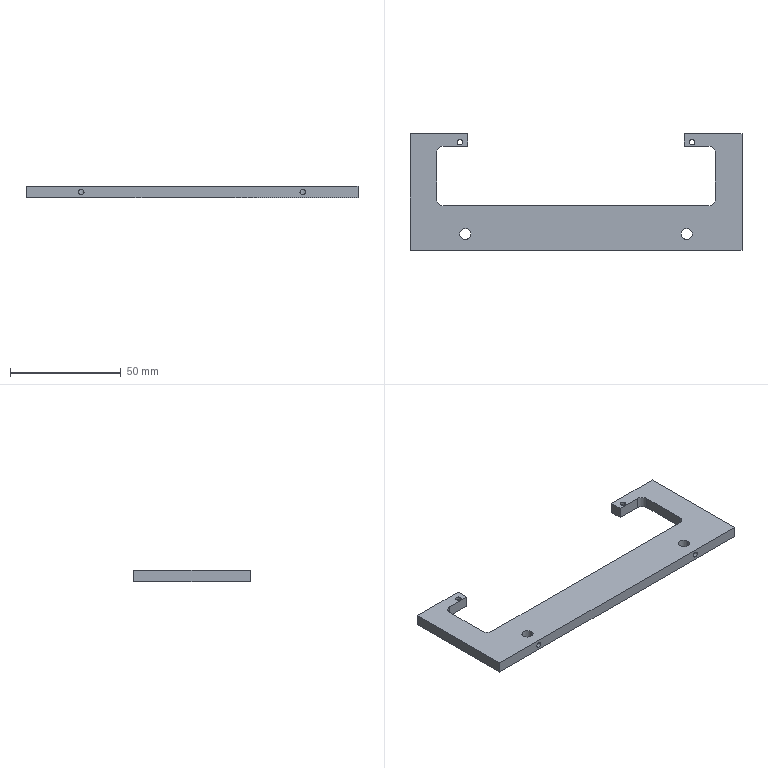Part | SolidWorks | features BaseBody 1 | 1 solid | 38 faces | box 150 x 52.5 x 5 mm | volume 19392 mm3 | cylinder 20 | plane 14 | cone 4 | commonest cylinder face diameters 2.459 x8 2.5 x4 5 x4 6 x4
STEP:
#1=CARTESIAN_POINT('',(104.953,41.271,5.));
#2=VERTEX_POINT('',#1);
#3=CARTESIAN_POINT('',(102.453,41.271,5.));
#4=VERTEX_POINT('',#3);
#5=CARTESIAN_POINT('',(103.703,41.271,5.));
#6=DIRECTION('',(0.,0.,-1.));
#7=DIRECTION('',(-1.,0.,0.));
#8=AXIS2_PLACEMENT_3D('',#5,#6,#7);
#9=CIRCLE('',#8,1.25);
#10=EDGE_CURVE('',#2,#4,#9,.T.);
#11=ORIENTED_EDGE('',*,*,#10,.F.);
#12=CARTESIAN_POINT('',(104.953,41.271,0.));
#13=VERTEX_POINT('',#12);
#14=CARTESIAN_POINT('',(104.953,41.271,158.352));
#15=DIRECTION('',(0.,0.,-1.));
#16=VECTOR('',#15,1000.);
#17=LINE('',#14,#16);
#18=EDGE_CURVE('',#2,#13,#17,.T.);
#19=ORIENTED_EDGE('',*,*,#18,.T.);
#20=CARTESIAN_POINT('',(102.453,41.271,0.));
#21=VERTEX_POINT('',#20);
#22=CARTESIAN_POINT('',(103.703,41.271,0.));
#23=DIRECTION('',(0.,0.,-1.));
#24=DIRECTION('',(-1.,0.,0.));
#25=AXIS2_PLACEMENT_3D('',#22,#23,#24);
#26=CIRCLE('',#25,1.25);
#27=EDGE_CURVE('',#13,#21,#26,.T.);
#28=ORIENTED_EDGE('',*,*,#27,.T.);
#29=CARTESIAN_POINT('',(102.453,41.271,158.352));
#30=DIRECTION('',(0.,0.,-1.));
#31=VECTOR('',#30,1000.);
#32=LINE('',#29,#31);
#33=EDGE_CURVE('',#4,#21,#32,.T.);
#34=ORIENTED_EDGE('',*,*,#33,.F.);
#35=EDGE_LOOP('',(#11,#19,#28,#34));
#36=FACE_OUTER_BOUND('',#35,.T.);
#37=CARTESIAN_POINT('',(103.703,41.271,158.352));
#38=DIRECTION('',(0.,0.,-1.));
#39=DIRECTION('',(-1.,0.,0.));
#40=AXIS2_PLACEMENT_3D('',#37,#38,#39);
#41=CYLINDRICAL_SURFACE('',#40,1.25);
#42=ADVANCED_FACE('',(#36),#41,.F.);
#43=CARTESIAN_POINT('',(-0.04679,41.271,5.));
#44=VERTEX_POINT('',#43);
#45=CARTESIAN_POINT('',(-2.547,41.271,5.));
#46=VERTEX_POINT('',#45);
#47=CARTESIAN_POINT('',(-1.297,41.271,5.));
#48=DIRECTION('',(0.,0.,-1.));
#49=DIRECTION('',(-1.,0.,0.));
#50=AXIS2_PLACEMENT_3D('',#47,#48,#49);
#51=CIRCLE('',#50,1.25);
#52=EDGE_CURVE('',#44,#46,#51,.T.);
#53=ORIENTED_EDGE('',*,*,#52,.F.);
#54=CARTESIAN_POINT('',(-0.04679,41.271,0.));
#55=VERTEX_POINT('',#54);
#56=CARTESIAN_POINT('',(-0.04679,41.271,158.352));
#57=DIRECTION('',(0.,0.,-1.));
#58=VECTOR('',#57,1000.);
#59=LINE('',#56,#58);
#60=EDGE_CURVE('',#44,#55,#59,.T.);
#61=ORIENTED_EDGE('',*,*,#60,.T.);
#62=CARTESIAN_POINT('',(-2.547,41.271,0.));
#63=VERTEX_POINT('',#62);
#64=CARTESIAN_POINT('',(-1.297,41.271,0.));
#65=DIRECTION('',(0.,0.,-1.));
#66=DIRECTION('',(-1.,0.,0.));
#67=AXIS2_PLACEMENT_3D('',#64,#65,#66);
#68=CIRCLE('',#67,1.25);
#69=EDGE_CURVE('',#55,#63,#68,.T.);
#70=ORIENTED_EDGE('',*,*,#69,.T.);
#71=CARTESIAN_POINT('',(-2.547,41.271,158.352));
#72=DIRECTION('',(0.,0.,-1.));
#73=VECTOR('',#72,1000.);
#74=LINE('',#71,#73);
#75=EDGE_CURVE('',#46,#63,#74,.T.);
#76=ORIENTED_EDGE('',*,*,#75,.F.);
#77=EDGE_LOOP('',(#53,#61,#70,#76));
#78=FACE_OUTER_BOUND('',#77,.T.);
#79=CARTESIAN_POINT('',(-1.297,41.271,158.352));
#80=DIRECTION('',(0.,0.,-1.));
#81=DIRECTION('',(-1.,0.,0.));
#82=AXIS2_PLACEMENT_3D('',#79,#80,#81);
#83=CYLINDRICAL_SURFACE('',#82,1.25);
#84=ADVANCED_FACE('',(#78),#83,.F.);
#85=CARTESIAN_POINT('',(102.433,-2.406,2.5));
#86=VERTEX_POINT('',#85);
#87=CARTESIAN_POINT('',(99.974,-2.406,2.5));
#88=VERTEX_POINT('',#87);
#89=CARTESIAN_POINT('',(102.433,-2.406,2.5));
#90=CARTESIAN_POINT('',(102.433,-2.406,2.419));
#91=CARTESIAN_POINT('',(102.424,-2.41,2.336));
#92=CARTESIAN_POINT('',(102.392,-2.428,2.177));
#93=CARTESIAN_POINT('',(102.368,-2.441,2.1));
#94=CARTESIAN_POINT('',(102.275,-2.489,1.876));
#95=CARTESIAN_POINT('',(102.184,-2.531,1.742));
#96=CARTESIAN_POINT('',(101.961,-2.614,1.519));
#97=CARTESIAN_POINT('',(101.826,-2.655,1.428));
#98=CARTESIAN_POINT('',(101.531,-2.712,1.304));
#99=CARTESIAN_POINT('',(101.367,-2.729,1.271));
#100=CARTESIAN_POINT('',(101.041,-2.729,1.27));
#101=CARTESIAN_POINT('',(100.878,-2.712,1.303));
#102=CARTESIAN_POINT('',(100.58,-2.655,1.428));
#103=CARTESIAN_POINT('',(100.446,-2.614,1.519));
#104=CARTESIAN_POINT('',(100.277,-2.552,1.687));
#105=CARTESIAN_POINT('',(100.227,-2.531,1.748));
#106=CARTESIAN_POINT('',(100.139,-2.492,1.88));
#107=CARTESIAN_POINT('',(100.1,-2.473,1.951));
#108=CARTESIAN_POINT('',(100.038,-2.441,2.099));
#109=CARTESIAN_POINT('',(100.015,-2.428,2.175));
#110=CARTESIAN_POINT('',(99.982,-2.411,2.334));
#111=CARTESIAN_POINT('',(99.974,-2.406,2.417));
#112=CARTESIAN_POINT('',(99.974,-2.406,2.5));
#113=B_SPLINE_CURVE_WITH_KNOTS('',3,(#89,#90,#91,#92,#93,#94,#95,#96,#97,#98,#99,#100,#101,#102,#103,#104,#105,#106,#107,#108,#109,#110,#111,#112),.UNSPECIFIED.,.F.,.F.,(4,2,2,2,2,2,2,2,2,2,2,4),(0.003908,0.004152,0.004396,0.004884,0.005371,0.005859,0.006347,0.006834,0.007078,0.007322,0.007566,0.00781),.UNSPECIFIED.);
#114=EDGE_CURVE('',#86,#88,#113,.T.);
#115=ORIENTED_EDGE('',*,*,#114,.F.);
#116=CARTESIAN_POINT('',(99.974,-2.406,2.5));
#117=CARTESIAN_POINT('',(99.974,-2.406,2.583));
#118=CARTESIAN_POINT('',(99.982,-2.41,2.664));
#119=CARTESIAN_POINT('',(100.014,-2.428,2.823));
#120=CARTESIAN_POINT('',(100.038,-2.441,2.901));
#121=CARTESIAN_POINT('',(100.131,-2.489,3.123));
#122=CARTESIAN_POINT('',(100.222,-2.531,3.258));
#123=CARTESIAN_POINT('',(100.445,-2.614,3.481));
#124=CARTESIAN_POINT('',(100.58,-2.655,3.572));
#125=CARTESIAN_POINT('',(100.801,-2.698,3.665));
#126=CARTESIAN_POINT('',(100.88,-2.709,3.689));
#127=CARTESIAN_POINT('',(101.04,-2.725,3.721));
#128=CARTESIAN_POINT('',(101.121,-2.729,3.729));
#129=CARTESIAN_POINT('',(101.366,-2.729,3.73));
#130=CARTESIAN_POINT('',(101.53,-2.712,3.696));
#131=CARTESIAN_POINT('',(101.828,-2.654,3.571));
#132=CARTESIAN_POINT('',(101.962,-2.614,3.48));
#133=CARTESIAN_POINT('',(102.185,-2.531,3.256));
#134=CARTESIAN_POINT('',(102.276,-2.488,3.121));
#135=CARTESIAN_POINT('',(102.399,-2.425,2.827));
#136=CARTESIAN_POINT('',(102.433,-2.406,2.663));
#137=CARTESIAN_POINT('',(102.433,-2.406,2.5));
#138=B_SPLINE_CURVE_WITH_KNOTS('',3,(#116,#117,#118,#119,#120,#121,#122,#123,#124,#125,#126,#127,#128,#129,#130,#131,#132,#133,#134,#135,#136,#137),.UNSPECIFIED.,.F.,.F.,(4,2,2,2,2,2,2,2,2,2,4),(0.,0.0002443,0.0004885,0.000977,0.001466,0.00171,0.001954,0.002443,0.002931,0.00342,0.003908),.UNSPECIFIED.);
#139=EDGE_CURVE('',#88,#86,#138,.T.);
#140=ORIENTED_EDGE('',*,*,#139,.F.);
#141=EDGE_LOOP('',(#115,#140));
#142=FACE_BOUND('',#141,.T.);
#143=CARTESIAN_POINT('',(103.703,-0.229,5.));
#144=VERTEX_POINT('',#143);
#145=CARTESIAN_POINT('',(98.703,-0.229,5.));
#146=VERTEX_POINT('',#145);
#147=CARTESIAN_POINT('',(101.203,-0.229,5.));
#148=DIRECTION('',(0.,0.,-1.));
#149=DIRECTION('',(-1.,0.,0.));
#150=AXIS2_PLACEMENT_3D('',#147,#148,#149);
#151=CIRCLE('',#150,2.5);
#152=EDGE_CURVE('',#144,#146,#151,.T.);
#153=ORIENTED_EDGE('',*,*,#152,.F.);
#154=CARTESIAN_POINT('',(103.703,-0.229,0.));
#155=VERTEX_POINT('',#154);
#156=CARTESIAN_POINT('',(103.703,-0.229,158.352));
#157=DIRECTION('',(0.,0.,-1.));
#158=VECTOR('',#157,1000.);
#159=LINE('',#156,#158);
#160=EDGE_CURVE('',#144,#155,#159,.T.);
#161=ORIENTED_EDGE('',*,*,#160,.T.);
#162=CARTESIAN_POINT('',(98.703,-0.229,0.));
#163=VERTEX_POINT('',#162);
#164=CARTESIAN_POINT('',(101.203,-0.229,0.));
#165=DIRECTION('',(0.,0.,-1.));
#166=DIRECTION('',(-1.,0.,0.));
#167=AXIS2_PLACEMENT_3D('',#164,#165,#166);
#168=CIRCLE('',#167,2.5);
#169=EDGE_CURVE('',#155,#163,#168,.T.);
#170=ORIENTED_EDGE('',*,*,#169,.T.);
#171=CARTESIAN_POINT('',(98.703,-0.229,158.352));
#172=DIRECTION('',(0.,0.,-1.));
#173=VECTOR('',#172,1000.);
#174=LINE('',#171,#173);
#175=EDGE_CURVE('',#146,#163,#174,.T.);
#176=ORIENTED_EDGE('',*,*,#175,.F.);
#177=EDGE_LOOP('',(#153,#161,#170,#176));
#178=FACE_OUTER_BOUND('',#177,.T.);
#179=CARTESIAN_POINT('',(101.203,-0.229,158.352));
#180=DIRECTION('',(0.,0.,-1.));
#181=DIRECTION('',(-1.,0.,0.));
#182=AXIS2_PLACEMENT_3D('',#179,#180,#181);
#183=CYLINDRICAL_SURFACE('',#182,2.5);
#184=ADVANCED_FACE('',(#142,#178),#183,.F.);
#185=CARTESIAN_POINT('',(2.433,-2.406,2.5));
#186=VERTEX_POINT('',#185);
#187=CARTESIAN_POINT('',(-0.02629,-2.406,2.5));
#188=VERTEX_POINT('',#187);
#189=CARTESIAN_POINT('',(2.433,-2.406,2.5));
#190=CARTESIAN_POINT('',(2.433,-2.406,2.419));
#191=CARTESIAN_POINT('',(2.424,-2.41,2.336));
#192=CARTESIAN_POINT('',(2.392,-2.428,2.177));
#193=CARTESIAN_POINT('',(2.368,-2.441,2.1));
#194=CARTESIAN_POINT('',(2.275,-2.489,1.876));
#195=CARTESIAN_POINT('',(2.184,-2.531,1.742));
#196=CARTESIAN_POINT('',(1.961,-2.614,1.519));
#197=CARTESIAN_POINT('',(1.826,-2.655,1.428));
#198=CARTESIAN_POINT('',(1.531,-2.712,1.304));
#199=CARTESIAN_POINT('',(1.367,-2.729,1.271));
#200=CARTESIAN_POINT('',(1.041,-2.729,1.27));
#201=CARTESIAN_POINT('',(0.8776,-2.712,1.303));
#202=CARTESIAN_POINT('',(0.5797,-2.655,1.428));
#203=CARTESIAN_POINT('',(0.4456,-2.614,1.519));
#204=CARTESIAN_POINT('',(0.277,-2.552,1.687));
#205=CARTESIAN_POINT('',(0.227,-2.531,1.748));
#206=CARTESIAN_POINT('',(0.1387,-2.492,1.88));
#207=CARTESIAN_POINT('',(0.1001,-2.473,1.951));
#208=CARTESIAN_POINT('',(0.03824,-2.441,2.099));
#209=CARTESIAN_POINT('',(0.01456,-2.428,2.175));
#210=CARTESIAN_POINT('',(-0.01779,-2.411,2.334));
#211=CARTESIAN_POINT('',(-0.02629,-2.406,2.417));
#212=CARTESIAN_POINT('',(-0.02629,-2.406,2.5));
#213=B_SPLINE_CURVE_WITH_KNOTS('',3,(#189,#190,#191,#192,#193,#194,#195,#196,#197,#198,#199,#200,#201,#202,#203,#204,#205,#206,#207,#208,#209,#210,#211,#212),.UNSPECIFIED.,.F.,.F.,(4,2,2,2,2,2,2,2,2,2,2,4),(0.003908,0.004152,0.004396,0.004884,0.005371,0.005859,0.006347,0.006834,0.007078,0.007322,0.007566,0.00781),.UNSPECIFIED.);
#214=EDGE_CURVE('',#186,#188,#213,.T.);
#215=ORIENTED_EDGE('',*,*,#214,.F.);
#216=CARTESIAN_POINT('',(-0.02629,-2.406,2.5));
#217=CARTESIAN_POINT('',(-0.02629,-2.406,2.583));
#218=CARTESIAN_POINT('',(-0.01803,-2.41,2.664));
#219=CARTESIAN_POINT('',(0.01402,-2.428,2.823));
#220=CARTESIAN_POINT('',(0.03825,-2.441,2.901));
#221=CARTESIAN_POINT('',(0.1313,-2.489,3.123));
#222=CARTESIAN_POINT('',(0.222,-2.531,3.258));
#223=CARTESIAN_POINT('',(0.445,-2.614,3.481));
#224=CARTESIAN_POINT('',(0.5798,-2.655,3.572));
#225=CARTESIAN_POINT('',(0.8014,-2.698,3.665));
#226=CARTESIAN_POINT('',(0.8802,-2.709,3.689));
#227=CARTESIAN_POINT('',(1.04,-2.725,3.721));
#228=CARTESIAN_POINT('',(1.121,-2.729,3.729));
#229=CARTESIAN_POINT('',(1.366,-2.729,3.73));
#230=CARTESIAN_POINT('',(1.53,-2.712,3.696));
#231=CARTESIAN_POINT('',(1.828,-2.654,3.571));
#232=CARTESIAN_POINT('',(1.962,-2.614,3.48));
#233=CARTESIAN_POINT('',(2.185,-2.531,3.256));
#234=CARTESIAN_POINT('',(2.276,-2.488,3.121));
#235=CARTESIAN_POINT('',(2.399,-2.425,2.827));
#236=CARTESIAN_POINT('',(2.433,-2.406,2.663));
#237=CARTESIAN_POINT('',(2.433,-2.406,2.5));
#238=B_SPLINE_CURVE_WITH_KNOTS('',3,(#216,#217,#218,#219,#220,#221,#222,#223,#224,#225,#226,#227,#228,#229,#230,#231,#232,#233,#234,#235,#236,#237),.UNSPECIFIED.,.F.,.F.,(4,2,2,2,2,2,2,2,2,2,4),(0.,0.0002443,0.0004885,0.000977,0.001466,0.00171,0.001954,0.002443,0.002931,0.00342,0.003908),.UNSPECIFIED.);
#239=EDGE_CURVE('',#188,#186,#238,.T.);
#240=ORIENTED_EDGE('',*,*,#239,.F.);
#241=EDGE_LOOP('',(#215,#240));
#242=FACE_BOUND('',#241,.T.);
#243=CARTESIAN_POINT('',(3.703,-0.229,5.));
#244=VERTEX_POINT('',#243);
#245=CARTESIAN_POINT('',(-1.297,-0.229,5.));
#246=VERTEX_POINT('',#245);
#247=CARTESIAN_POINT('',(1.203,-0.229,5.));
#248=DIRECTION('',(0.,0.,-1.));
#249=DIRECTION('',(-1.,0.,0.));
#250=AXIS2_PLACEMENT_3D('',#247,#248,#249);
#251=CIRCLE('',#250,2.5);
#252=EDGE_CURVE('',#244,#246,#251,.T.);
#253=ORIENTED_EDGE('',*,*,#252,.F.);
#254=CARTESIAN_POINT('',(3.703,-0.229,0.));
#255=VERTEX_POINT('',#254);
#256=CARTESIAN_POINT('',(3.703,-0.229,158.352));
#257=DIRECTION('',(0.,0.,-1.));
#258=VECTOR('',#257,1000.);
#259=LINE('',#256,#258);
#260=EDGE_CURVE('',#244,#255,#259,.T.);
#261=ORIENTED_EDGE('',*,*,#260,.T.);
#262=CARTESIAN_POINT('',(-1.297,-0.229,0.));
#263=VERTEX_POINT('',#262);
#264=CARTESIAN_POINT('',(1.203,-0.229,0.));
#265=DIRECTION('',(0.,0.,-1.));
#266=DIRECTION('',(-1.,0.,0.));
#267=AXIS2_PLACEMENT_3D('',#264,#265,#266);
#268=CIRCLE('',#267,2.5);
#269=EDGE_CURVE('',#255,#263,#268,.T.);
#270=ORIENTED_EDGE('',*,*,#269,.T.);
#271=CARTESIAN_POINT('',(-1.297,-0.229,158.352));
#272=DIRECTION('',(0.,0.,-1.));
#273=VECTOR('',#272,1000.);
#274=LINE('',#271,#273);
#275=EDGE_CURVE('',#246,#263,#274,.T.);
#276=ORIENTED_EDGE('',*,*,#275,.F.);
#277=EDGE_LOOP('',(#253,#261,#270,#276));
#278=FACE_OUTER_BOUND('',#277,.T.);
#279=CARTESIAN_POINT('',(1.203,-0.229,158.352));
#280=DIRECTION('',(0.,0.,-1.));
#281=DIRECTION('',(-1.,0.,0.));
#282=AXIS2_PLACEMENT_3D('',#279,#280,#281);
#283=CYLINDRICAL_SURFACE('',#282,2.5);
#284=ADVANCED_FACE('',(#242,#278),#283,.F.);
#285=CARTESIAN_POINT('',(104.933,42.021,2.5));
#286=VERTEX_POINT('',#285);
#287=CARTESIAN_POINT('',(104.703,42.021,1.785));
#288=VERTEX_POINT('',#287);
#289=CARTESIAN_POINT('',(103.703,42.021,2.5));
#290=DIRECTION('',(0.,1.,0.));
#291=DIRECTION('',(-1.,0.,0.));
#292=AXIS2_PLACEMENT_3D('',#289,#290,#291);
#293=CIRCLE('',#292,1.229);
#294=EDGE_CURVE('',#286,#288,#293,.T.);
#295=ORIENTED_EDGE('',*,*,#294,.F.);
#296=CARTESIAN_POINT('',(104.933,45.021,2.5));
#297=VERTEX_POINT('',#296);
#298=CARTESIAN_POINT('',(104.933,43.521,2.5));
#299=DIRECTION('',(0.,1.,0.));
#300=VECTOR('',#299,1000.);
#301=LINE('',#298,#300);
#302=EDGE_CURVE('',#286,#297,#301,.T.);
#303=ORIENTED_EDGE('',*,*,#302,.T.);
#304=CARTESIAN_POINT('',(102.474,45.021,2.5));
#305=VERTEX_POINT('',#304);
#306=CARTESIAN_POINT('',(103.703,45.021,2.5));
#307=DIRECTION('',(0.,-1.,0.));
#308=DIRECTION('',(-1.,0.,0.));
#309=AXIS2_PLACEMENT_3D('',#306,#307,#308);
#310=CIRCLE('',#309,1.229);
#311=EDGE_CURVE('',#305,#297,#310,.T.);
#312=ORIENTED_EDGE('',*,*,#311,.F.);
#313=CARTESIAN_POINT('',(102.474,42.021,2.5));
#314=VERTEX_POINT('',#313);
#315=CARTESIAN_POINT('',(102.474,43.521,2.5));
#316=DIRECTION('',(0.,1.,0.));
#317=VECTOR('',#316,1000.);
#318=LINE('',#315,#317);
#319=EDGE_CURVE('',#314,#305,#318,.T.);
#320=ORIENTED_EDGE('',*,*,#319,.F.);
#321=CARTESIAN_POINT('',(102.703,42.021,1.785));
#322=VERTEX_POINT('',#321);
#323=CARTESIAN_POINT('',(103.703,42.021,2.5));
#324=DIRECTION('',(0.,-1.,0.));
#325=DIRECTION('',(1.,0.,0.));
#326=AXIS2_PLACEMENT_3D('',#323,#324,#325);
#327=CIRCLE('',#326,1.229);
#328=EDGE_CURVE('',#314,#322,#327,.T.);
#329=ORIENTED_EDGE('',*,*,#328,.T.);
#330=CARTESIAN_POINT('',(102.703,42.021,1.785));
#331=CARTESIAN_POINT('',(102.753,42.087,1.715));
#332=CARTESIAN_POINT('',(102.81,42.15,1.65));
#333=CARTESIAN_POINT('',(102.943,42.268,1.529));
#334=CARTESIAN_POINT('',(103.02,42.322,1.473));
#335=CARTESIAN_POINT('',(103.19,42.415,1.379));
#336=CARTESIAN_POINT('',(103.285,42.453,1.339));
#337=CARTESIAN_POINT('',(103.486,42.507,1.285));
#338=CARTESIAN_POINT('',(103.595,42.521,1.271));
#339=CARTESIAN_POINT('',(103.81,42.521,1.27));
#340=CARTESIAN_POINT('',(103.918,42.507,1.285));
#341=CARTESIAN_POINT('',(104.12,42.454,1.339));
#342=CARTESIAN_POINT('',(104.216,42.415,1.378));
#343=CARTESIAN_POINT('',(104.47,42.277,1.52));
#344=CARTESIAN_POINT('',(104.603,42.154,1.645));
#345=CARTESIAN_POINT('',(104.703,42.021,1.785));
#346=B_SPLINE_CURVE_WITH_KNOTS('',3,(#330,#331,#332,#333,#334,#335,#336,#337,#338,#339,#340,#341,#342,#343,#344,#345),.UNSPECIFIED.,.F.,.F.,(4,2,2,2,2,2,2,4),(0.,0.0003213,0.0006427,0.000964,0.001285,0.001607,0.001928,0.002571),.UNSPECIFIED.);
#347=EDGE_CURVE('',#322,#288,#346,.T.);
#348=ORIENTED_EDGE('',*,*,#347,.T.);
#349=EDGE_LOOP('',(#295,#303,#312,#320,#329,#348));
#350=FACE_OUTER_BOUND('',#349,.T.);
#351=CARTESIAN_POINT('',(103.703,43.521,2.5));
#352=DIRECTION('',(0.,1.,0.));
#353=DIRECTION('',(-1.,0.,0.));
#354=AXIS2_PLACEMENT_3D('',#351,#352,#353);
#355=CYLINDRICAL_SURFACE('',#354,1.229);
#356=ADVANCED_FACE('',(#350),#355,.F.);
#357=CARTESIAN_POINT('',(-0.06729,42.021,2.5));
#358=VERTEX_POINT('',#357);
#359=CARTESIAN_POINT('',(-0.2968,42.021,1.785));
#360=VERTEX_POINT('',#359);
#361=CARTESIAN_POINT('',(-1.297,42.021,2.5));
#362=DIRECTION('',(0.,1.,0.));
#363=DIRECTION('',(-1.,0.,0.));
#364=AXIS2_PLACEMENT_3D('',#361,#362,#363);
#365=CIRCLE('',#364,1.23);
#366=EDGE_CURVE('',#358,#360,#365,.T.);
#367=ORIENTED_EDGE('',*,*,#366,.F.);
#368=CARTESIAN_POINT('',(-0.06729,45.021,2.5));
#369=VERTEX_POINT('',#368);
#370=CARTESIAN_POINT('',(-0.06729,43.521,2.5));
#371=DIRECTION('',(0.,1.,0.));
#372=VECTOR('',#371,1000.);
#373=LINE('',#370,#372);
#374=EDGE_CURVE('',#358,#369,#373,.T.);
#375=ORIENTED_EDGE('',*,*,#374,.T.);
#376=CARTESIAN_POINT('',(-2.526,45.021,2.5));
#377=VERTEX_POINT('',#376);
#378=CARTESIAN_POINT('',(-1.297,45.021,2.5));
#379=DIRECTION('',(0.,-1.,0.));
#380=DIRECTION('',(-1.,0.,0.));
#381=AXIS2_PLACEMENT_3D('',#378,#379,#380);
#382=CIRCLE('',#381,1.23);
#383=EDGE_CURVE('',#377,#369,#382,.T.);
#384=ORIENTED_EDGE('',*,*,#383,.F.);
#385=CARTESIAN_POINT('',(-2.526,42.021,2.5));
#386=VERTEX_POINT('',#385);
#387=CARTESIAN_POINT('',(-2.526,43.521,2.5));
#388=DIRECTION('',(0.,1.,0.));
#389=VECTOR('',#388,1000.);
#390=LINE('',#387,#389);
#391=EDGE_CURVE('',#386,#377,#390,.T.);
#392=ORIENTED_EDGE('',*,*,#391,.F.);
#393=CARTESIAN_POINT('',(-2.297,42.021,1.785));
#394=VERTEX_POINT('',#393);
#395=CARTESIAN_POINT('',(-1.297,42.021,2.5));
#396=DIRECTION('',(0.,-1.,0.));
#397=DIRECTION('',(1.,0.,0.));
#398=AXIS2_PLACEMENT_3D('',#395,#396,#397);
#399=CIRCLE('',#398,1.229);
#400=EDGE_CURVE('',#386,#394,#399,.T.);
#401=ORIENTED_EDGE('',*,*,#400,.T.);
#402=CARTESIAN_POINT('',(-2.297,42.021,1.785));
#403=CARTESIAN_POINT('',(-2.247,42.087,1.715));
#404=CARTESIAN_POINT('',(-2.19,42.15,1.65));
#405=CARTESIAN_POINT('',(-2.057,42.268,1.529));
#406=CARTESIAN_POINT('',(-1.98,42.322,1.473));
#407=CARTESIAN_POINT('',(-1.81,42.415,1.379));
#408=CARTESIAN_POINT('',(-1.715,42.453,1.339));
#409=CARTESIAN_POINT('',(-1.514,42.507,1.285));
#410=CARTESIAN_POINT('',(-1.405,42.521,1.271));
#411=CARTESIAN_POINT('',(-1.19,42.521,1.27));
#412=CARTESIAN_POINT('',(-1.082,42.507,1.285));
#413=CARTESIAN_POINT('',(-0.8797,42.454,1.339));
#414=CARTESIAN_POINT('',(-0.7845,42.415,1.378));
#415=CARTESIAN_POINT('',(-0.53,42.277,1.52));
#416=CARTESIAN_POINT('',(-0.3965,42.154,1.645));
#417=CARTESIAN_POINT('',(-0.2968,42.021,1.785));
#418=B_SPLINE_CURVE_WITH_KNOTS('',3,(#402,#403,#404,#405,#406,#407,#408,#409,#410,#411,#412,#413,#414,#415,#416,#417),.UNSPECIFIED.,.F.,.F.,(4,2,2,2,2,2,2,4),(0.,0.0003213,0.0006427,0.000964,0.001285,0.001607,0.001928,0.002571),.UNSPECIFIED.);
#419=EDGE_CURVE('',#394,#360,#418,.T.);
#420=ORIENTED_EDGE('',*,*,#419,.T.);
#421=EDGE_LOOP('',(#367,#375,#384,#392,#401,#420));
#422=FACE_OUTER_BOUND('',#421,.T.);
#423=CARTESIAN_POINT('',(-1.297,43.521,2.5));
#424=DIRECTION('',(0.,1.,0.));
#425=DIRECTION('',(-1.,0.,0.));
#426=AXIS2_PLACEMENT_3D('',#423,#424,#425);
#427=CYLINDRICAL_SURFACE('',#426,1.23);
#428=ADVANCED_FACE('',(#422),#427,.F.);
#429=ORIENTED_EDGE('',*,*,#114,.T.);
#430=CARTESIAN_POINT('',(99.974,-7.479,2.5));
#431=VERTEX_POINT('',#430);
#432=CARTESIAN_POINT('',(99.974,-3.979,2.5));
#433=DIRECTION('',(0.,-1.,0.));
#434=VECTOR('',#433,1000.);
#435=LINE('',#432,#434);
#436=EDGE_CURVE('',#88,#431,#435,.T.);
#437=ORIENTED_EDGE('',*,*,#436,.T.);
#438=CARTESIAN_POINT('',(102.433,-7.479,2.5));
#439=VERTEX_POINT('',#438);
#440=CARTESIAN_POINT('',(101.203,-7.479,2.5));
#441=DIRECTION('',(0.,1.,0.));
#442=DIRECTION('',(1.,0.,0.));
#443=AXIS2_PLACEMENT_3D('',#440,#441,#442);
#444=CIRCLE('',#443,1.229);
#445=EDGE_CURVE('',#439,#431,#444,.T.);
#446=ORIENTED_EDGE('',*,*,#445,.F.);
#447=CARTESIAN_POINT('',(102.433,-3.979,2.5));
#448=DIRECTION('',(0.,-1.,0.));
#449=VECTOR('',#448,1000.);
#450=LINE('',#447,#449);
#451=EDGE_CURVE('',#86,#439,#450,.T.);
#452=ORIENTED_EDGE('',*,*,#451,.F.);
#453=EDGE_LOOP('',(#429,#437,#446,#452));
#454=FACE_OUTER_BOUND('',#453,.T.);
#455=CARTESIAN_POINT('',(101.203,-3.979,2.5));
#456=DIRECTION('',(0.,-1.,0.));
#457=DIRECTION('',(1.,0.,0.));
#458=AXIS2_PLACEMENT_3D('',#455,#456,#457);
#459=CYLINDRICAL_SURFACE('',#458,1.229);
#460=ADVANCED_FACE('',(#454),#459,.F.);
#461=ORIENTED_EDGE('',*,*,#214,.T.);
#462=CARTESIAN_POINT('',(-0.02629,-7.479,2.5));
#463=VERTEX_POINT('',#462);
#464=CARTESIAN_POINT('',(-0.02629,-3.979,2.5));
#465=DIRECTION('',(0.,-1.,0.));
#466=VECTOR('',#465,1000.);
#467=LINE('',#464,#466);
#468=EDGE_CURVE('',#188,#463,#467,.T.);
#469=ORIENTED_EDGE('',*,*,#468,.T.);
#470=CARTESIAN_POINT('',(2.433,-7.479,2.5));
#471=VERTEX_POINT('',#470);
#472=CARTESIAN_POINT('',(1.203,-7.479,2.5));
#473=DIRECTION('',(0.,1.,0.));
#474=DIRECTION('',(1.,0.,0.));
#475=AXIS2_PLACEMENT_3D('',#472,#473,#474);
#476=CIRCLE('',#475,1.23);
#477=EDGE_CURVE('',#471,#463,#476,.T.);
#478=ORIENTED_EDGE('',*,*,#477,.F.);
#479=CARTESIAN_POINT('',(2.433,-3.979,2.5));
#480=DIRECTION('',(0.,-1.,0.));
#481=VECTOR('',#480,1000.);
#482=LINE('',#479,#481);
#483=EDGE_CURVE('',#186,#471,#482,.T.);
#484=ORIENTED_EDGE('',*,*,#483,.F.);
#485=EDGE_LOOP('',(#461,#469,#478,#484));
#486=FACE_OUTER_BOUND('',#485,.T.);
#487=CARTESIAN_POINT('',(1.203,-3.979,2.5));
#488=DIRECTION('',(0.,-1.,0.));
#489=DIRECTION('',(1.,0.,0.));
#490=AXIS2_PLACEMENT_3D('',#487,#488,#489);
#491=CYLINDRICAL_SURFACE('',#490,1.23);
#492=ADVANCED_FACE('',(#486),#491,.F.);
#493=CARTESIAN_POINT('',(103.703,41.271,0.));
#494=DIRECTION('',(0.,0.,-1.));
#495=DIRECTION('',(-1.,0.,0.));
#496=AXIS2_PLACEMENT_3D('',#493,#494,#495);
#497=CIRCLE('',#496,1.25);
#498=EDGE_CURVE('',#21,#13,#497,.T.);
#499=ORIENTED_EDGE('',*,*,#498,.F.);
#500=ORIENTED_EDGE('',*,*,#27,.F.);
#501=EDGE_LOOP('',(#499,#500));
#502=FACE_BOUND('',#501,.T.);
#503=CARTESIAN_POINT('',(-1.297,41.271,0.));
#504=DIRECTION('',(0.,0.,-1.));
#505=DIRECTION('',(-1.,0.,0.));
#506=AXIS2_PLACEMENT_3D('',#503,#504,#505);
#507=CIRCLE('',#506,1.25);
#508=EDGE_CURVE('',#63,#55,#507,.T.);
#509=ORIENTED_EDGE('',*,*,#508,.F.);
#510=ORIENTED_EDGE('',*,*,#69,.F.);
#511=EDGE_LOOP('',(#509,#510));
#512=FACE_BOUND('',#511,.T.);
#513=CARTESIAN_POINT('',(101.203,-0.229,0.));
#514=DIRECTION('',(0.,0.,-1.));
#515=DIRECTION('',(-1.,0.,0.));
#516=AXIS2_PLACEMENT_3D('',#513,#514,#515);
#517=CIRCLE('',#516,2.5);
#518=EDGE_CURVE('',#163,#155,#517,.T.);
#519=ORIENTED_EDGE('',*,*,#518,.F.);
#520=ORIENTED_EDGE('',*,*,#169,.F.);
#521=EDGE_LOOP('',(#519,#520));
#522=FACE_BOUND('',#521,.T.);
#523=CARTESIAN_POINT('',(1.203,-0.229,0.));
#524=DIRECTION('',(0.,0.,-1.));
#525=DIRECTION('',(-1.,0.,0.));
#526=AXIS2_PLACEMENT_3D('',#523,#524,#525);
#527=CIRCLE('',#526,2.5);
#528=EDGE_CURVE('',#263,#255,#527,.T.);
#529=ORIENTED_EDGE('',*,*,#528,.F.);
#530=ORIENTED_EDGE('',*,*,#269,.F.);
#531=EDGE_LOOP('',(#529,#530));
#532=FACE_BOUND('',#531,.T.);
#533=CARTESIAN_POINT('',(-8.797,39.521,0.));
#534=VERTEX_POINT('',#533);
#535=CARTESIAN_POINT('',(2.203,39.521,0.));
#536=VERTEX_POINT('',#535);
#537=CARTESIAN_POINT('',(-4.797,39.521,0.));
#538=DIRECTION('',(1.,0.,0.));
#539=VECTOR('',#538,1000.);
#540=LINE('',#537,#539);
#541=EDGE_CURVE('',#534,#536,#540,.T.);
#542=ORIENTED_EDGE('',*,*,#541,.F.);
#543=CARTESIAN_POINT('',(-11.797,36.521,0.));
#544=VERTEX_POINT('',#543);
#545=CARTESIAN_POINT('',(-8.797,36.521,0.));
#546=DIRECTION('',(0.,0.,-1.));
#547=DIRECTION('',(1.,0.,0.));
#548=AXIS2_PLACEMENT_3D('',#545,#546,#547);
#549=CIRCLE('',#548,3.);
#550=EDGE_CURVE('',#544,#534,#549,.T.);
#551=ORIENTED_EDGE('',*,*,#550,.F.);
#552=CARTESIAN_POINT('',(-11.797,15.521,0.));
#553=VERTEX_POINT('',#552);
#554=CARTESIAN_POINT('',(-11.797,41.271,0.));
#555=DIRECTION('',(0.,1.,0.));
#556=VECTOR('',#555,1000.);
#557=LINE('',#554,#556);
#558=EDGE_CURVE('',#553,#544,#557,.T.);
#559=ORIENTED_EDGE('',*,*,#558,.F.);
#560=CARTESIAN_POINT('',(-8.797,12.521,0.));
#561=VERTEX_POINT('',#560);
#562=CARTESIAN_POINT('',(-8.797,15.521,0.));
#563=DIRECTION('',(0.,0.,-1.));
#564=DIRECTION('',(1.,0.,0.));
#565=AXIS2_PLACEMENT_3D('',#562,#563,#564);
#566=CIRCLE('',#565,3.);
#567=EDGE_CURVE('',#561,#553,#566,.T.);
#568=ORIENTED_EDGE('',*,*,#567,.F.);
#569=CARTESIAN_POINT('',(111.203,12.521,0.));
#570=VERTEX_POINT('',#569);
#571=CARTESIAN_POINT('',(-4.797,12.521,0.));
#572=DIRECTION('',(-1.,0.,0.));
#573=VECTOR('',#572,1000.);
#574=LINE('',#571,#573);
#575=EDGE_CURVE('',#570,#561,#574,.T.);
#576=ORIENTED_EDGE('',*,*,#575,.F.);
#577=CARTESIAN_POINT('',(114.203,15.521,0.));
#578=VERTEX_POINT('',#577);
#579=CARTESIAN_POINT('',(111.203,15.521,0.));
#580=DIRECTION('',(0.,0.,-1.));
#581=DIRECTION('',(1.,0.,0.));
#582=AXIS2_PLACEMENT_3D('',#579,#580,#581);
#583=CIRCLE('',#582,3.);
#584=EDGE_CURVE('',#578,#570,#583,.T.);
#585=ORIENTED_EDGE('',*,*,#584,.F.);
#586=CARTESIAN_POINT('',(114.203,36.521,0.));
#587=VERTEX_POINT('',#586);
#588=CARTESIAN_POINT('',(114.203,41.271,0.));
#589=DIRECTION('',(0.,-1.,0.));
#590=VECTOR('',#589,1000.);
#591=LINE('',#588,#590);
#592=EDGE_CURVE('',#587,#578,#591,.T.);
#593=ORIENTED_EDGE('',*,*,#592,.F.);
#594=CARTESIAN_POINT('',(111.203,39.521,0.));
#595=VERTEX_POINT('',#594);
#596=CARTESIAN_POINT('',(111.203,36.521,0.));
#597=DIRECTION('',(0.,0.,-1.));
#598=DIRECTION('',(1.,0.,0.));
#599=AXIS2_PLACEMENT_3D('',#596,#597,#598);
#600=CIRCLE('',#599,3.);
#601=EDGE_CURVE('',#595,#587,#600,.T.);
#602=ORIENTED_EDGE('',*,*,#601,.F.);
#603=CARTESIAN_POINT('',(100.203,39.521,0.));
#604=VERTEX_POINT('',#603);
#605=CARTESIAN_POINT('',(-4.797,39.521,0.));
#606=DIRECTION('',(1.,0.,0.));
#607=VECTOR('',#606,1000.);
#608=LINE('',#605,#607);
#609=EDGE_CURVE('',#604,#595,#608,.T.);
#610=ORIENTED_EDGE('',*,*,#609,.F.);
#611=CARTESIAN_POINT('',(100.203,45.021,0.));
#612=VERTEX_POINT('',#611);
#613=CARTESIAN_POINT('',(100.203,41.271,0.));
#614=DIRECTION('',(0.,-1.,0.));
#615=VECTOR('',#614,1000.);
#616=LINE('',#613,#615);
#617=EDGE_CURVE('',#612,#604,#616,.T.);
#618=ORIENTED_EDGE('',*,*,#617,.F.);
#619=CARTESIAN_POINT('',(126.203,45.021,0.));
#620=VERTEX_POINT('',#619);
#621=CARTESIAN_POINT('',(-4.797,45.021,0.));
#622=DIRECTION('',(-1.,0.,0.));
#623=VECTOR('',#622,1000.);
#624=LINE('',#621,#623);
#625=EDGE_CURVE('',#620,#612,#624,.T.);
#626=ORIENTED_EDGE('',*,*,#625,.F.);
#627=CARTESIAN_POINT('',(126.203,-7.479,0.));
#628=VERTEX_POINT('',#627);
#629=CARTESIAN_POINT('',(126.203,41.271,0.));
#630=DIRECTION('',(0.,1.,0.));
#631=VECTOR('',#630,1000.);
#632=LINE('',#629,#631);
#633=EDGE_CURVE('',#628,#620,#632,.T.);
#634=ORIENTED_EDGE('',*,*,#633,.F.);
#635=CARTESIAN_POINT('',(-23.797,-7.479,0.));
#636=VERTEX_POINT('',#635);
#637=CARTESIAN_POINT('',(-4.797,-7.479,0.));
#638=DIRECTION('',(1.,0.,0.));
#639=VECTOR('',#638,1000.);
#640=LINE('',#637,#639);
#641=EDGE_CURVE('',#636,#628,#640,.T.);
#642=ORIENTED_EDGE('',*,*,#641,.F.);
#643=CARTESIAN_POINT('',(-23.797,45.021,0.));
#644=VERTEX_POINT('',#643);
#645=CARTESIAN_POINT('',(-23.797,41.271,0.));
#646=DIRECTION('',(0.,-1.,0.));
#647=VECTOR('',#646,1000.);
#648=LINE('',#645,#647);
#649=EDGE_CURVE('',#644,#636,#648,.T.);
#650=ORIENTED_EDGE('',*,*,#649,.F.);
#651=CARTESIAN_POINT('',(2.203,45.021,0.));
#652=VERTEX_POINT('',#651);
#653=CARTESIAN_POINT('',(-4.797,45.021,0.));
#654=DIRECTION('',(-1.,0.,0.));
#655=VECTOR('',#654,1000.);
#656=LINE('',#653,#655);
#657=EDGE_CURVE('',#652,#644,#656,.T.);
#658=ORIENTED_EDGE('',*,*,#657,.F.);
#659=CARTESIAN_POINT('',(2.203,41.271,0.));
#660=DIRECTION('',(0.,1.,0.));
#661=VECTOR('',#660,1000.);
#662=LINE('',#659,#661);
#663=EDGE_CURVE('',#536,#652,#662,.T.);
#664=ORIENTED_EDGE('',*,*,#663,.F.);
#665=EDGE_LOOP('',(#542,#551,#559,#568,#576,#585,#593,#602,#610,#618,#626,#634,#642,#650,#658,#664));
#666=FACE_OUTER_BOUND('',#665,.T.);
#667=CARTESIAN_POINT('',(-4.797,41.271,0.));
#668=DIRECTION('',(0.,0.,1.));
#669=DIRECTION('',(1.,0.,0.));
#670=AXIS2_PLACEMENT_3D('',#667,#668,#669);
#671=PLANE('',#670);
#672=ADVANCED_FACE('',(#502,#512,#522,#532,#666),#671,.F.);
#673=ORIENTED_EDGE('',*,*,#18,.F.);
#674=CARTESIAN_POINT('',(103.703,41.271,5.));
#675=DIRECTION('',(0.,0.,-1.));
#676=DIRECTION('',(-1.,0.,0.));
#677=AXIS2_PLACEMENT_3D('',#674,#675,#676);
#678=CIRCLE('',#677,1.25);
#679=EDGE_CURVE('',#4,#2,#678,.T.);
#680=ORIENTED_EDGE('',*,*,#679,.F.);
#681=ORIENTED_EDGE('',*,*,#33,.T.);
#682=ORIENTED_EDGE('',*,*,#498,.T.);
#683=EDGE_LOOP('',(#673,#680,#681,#682));
#684=FACE_OUTER_BOUND('',#683,.T.);
#685=CARTESIAN_POINT('',(104.703,42.021,3.215));
#686=VERTEX_POINT('',#685);
#687=CARTESIAN_POINT('',(102.703,42.021,3.215));
#688=VERTEX_POINT('',#687);
#689=CARTESIAN_POINT('',(104.703,42.021,3.215));
#690=CARTESIAN_POINT('',(104.653,42.087,3.285));
#691=CARTESIAN_POINT('',(104.596,42.15,3.35));
#692=CARTESIAN_POINT('',(104.463,42.268,3.471));
#693=CARTESIAN_POINT('',(104.386,42.322,3.527));
#694=CARTESIAN_POINT('',(104.217,42.415,3.621));
#695=CARTESIAN_POINT('',(104.122,42.453,3.661));
#696=CARTESIAN_POINT('',(103.92,42.507,3.715));
#697=CARTESIAN_POINT('',(103.812,42.521,3.729));
#698=CARTESIAN_POINT('',(103.596,42.521,3.73));
#699=CARTESIAN_POINT('',(103.488,42.507,3.715));
#700=CARTESIAN_POINT('',(103.286,42.454,3.661));
#701=CARTESIAN_POINT('',(103.191,42.415,3.622));
#702=CARTESIAN_POINT('',(102.936,42.277,3.48));
#703=CARTESIAN_POINT('',(102.803,42.154,3.355));
#704=CARTESIAN_POINT('',(102.703,42.021,3.215));
#705=B_SPLINE_CURVE_WITH_KNOTS('',3,(#689,#690,#691,#692,#693,#694,#695,#696,#697,#698,#699,#700,#701,#702,#703,#704),.UNSPECIFIED.,.F.,.F.,(4,2,2,2,2,2,2,4),(0.,0.0003213,0.0006427,0.000964,0.001285,0.001607,0.001928,0.002571),.UNSPECIFIED.);
#706=EDGE_CURVE('',#686,#688,#705,.T.);
#707=ORIENTED_EDGE('',*,*,#706,.F.);
#708=CARTESIAN_POINT('',(104.703,42.021,1.785));
#709=CARTESIAN_POINT('',(104.748,41.961,2.018));
#710=CARTESIAN_POINT('',(104.77,41.923,2.258));
#711=CARTESIAN_POINT('',(104.77,41.923,2.746));
#712=CARTESIAN_POINT('',(104.748,41.962,2.983));
#713=CARTESIAN_POINT('',(104.703,42.021,3.215));
#714=B_SPLINE_CURVE_WITH_KNOTS('',3,(#708,#709,#710,#711,#712,#713),.UNSPECIFIED.,.F.,.F.,(4,2,4),(0.,0.0007269,0.001454),.UNSPECIFIED.);
#715=EDGE_CURVE('',#288,#686,#714,.T.);
#716=ORIENTED_EDGE('',*,*,#715,.F.);
#717=ORIENTED_EDGE('',*,*,#347,.F.);
#718=CARTESIAN_POINT('',(102.703,42.021,3.215));
#719=CARTESIAN_POINT('',(102.659,41.961,2.982));
#720=CARTESIAN_POINT('',(102.637,41.923,2.742));
#721=CARTESIAN_POINT('',(102.637,41.923,2.254));
#722=CARTESIAN_POINT('',(102.659,41.962,2.017));
#723=CARTESIAN_POINT('',(102.703,42.021,1.785));
#724=B_SPLINE_CURVE_WITH_KNOTS('',3,(#718,#719,#720,#721,#722,#723),.UNSPECIFIED.,.F.,.F.,(4,2,4),(0.,0.0007269,0.001454),.UNSPECIFIED.);
#725=EDGE_CURVE('',#688,#322,#724,.T.);
#726=ORIENTED_EDGE('',*,*,#725,.F.);
#727=EDGE_LOOP('',(#707,#716,#717,#726));
#728=FACE_BOUND('',#727,.T.);
#729=CARTESIAN_POINT('',(103.703,41.271,158.352));
#730=DIRECTION('',(0.,0.,-1.));
#731=DIRECTION('',(-1.,0.,0.));
#732=AXIS2_PLACEMENT_3D('',#729,#730,#731);
#733=CYLINDRICAL_SURFACE('',#732,1.25);
#734=ADVANCED_FACE('',(#684,#728),#733,.F.);
#735=ORIENTED_EDGE('',*,*,#60,.F.);
#736=CARTESIAN_POINT('',(-1.297,41.271,5.));
#737=DIRECTION('',(0.,0.,-1.));
#738=DIRECTION('',(-1.,0.,0.));
#739=AXIS2_PLACEMENT_3D('',#736,#737,#738);
#740=CIRCLE('',#739,1.25);
#741=EDGE_CURVE('',#46,#44,#740,.T.);
#742=ORIENTED_EDGE('',*,*,#741,.F.);
#743=ORIENTED_EDGE('',*,*,#75,.T.);
#744=ORIENTED_EDGE('',*,*,#508,.T.);
#745=EDGE_LOOP('',(#735,#742,#743,#744));
#746=FACE_OUTER_BOUND('',#745,.T.);
#747=CARTESIAN_POINT('',(-0.2968,42.021,3.215));
#748=VERTEX_POINT('',#747);
#749=CARTESIAN_POINT('',(-2.297,42.021,3.215));
#750=VERTEX_POINT('',#749);
#751=CARTESIAN_POINT('',(-0.2968,42.021,3.215));
#752=CARTESIAN_POINT('',(-0.3466,42.087,3.285));
#753=CARTESIAN_POINT('',(-0.4041,42.15,3.35));
#754=CARTESIAN_POINT('',(-0.537,42.268,3.471));
#755=CARTESIAN_POINT('',(-0.6137,42.322,3.527));
#756=CARTESIAN_POINT('',(-0.7834,42.415,3.621));
#757=CARTESIAN_POINT('',(-0.8782,42.453,3.661));
#758=CARTESIAN_POINT('',(-1.08,42.507,3.715));
#759=CARTESIAN_POINT('',(-1.188,42.521,3.729));
#760=CARTESIAN_POINT('',(-1.404,42.521,3.73));
#761=CARTESIAN_POINT('',(-1.512,42.507,3.715));
#762=CARTESIAN_POINT('',(-1.714,42.454,3.661));
#763=CARTESIAN_POINT('',(-1.809,42.415,3.622));
#764=CARTESIAN_POINT('',(-2.064,42.277,3.48));
#765=CARTESIAN_POINT('',(-2.197,42.154,3.355));
#766=CARTESIAN_POINT('',(-2.297,42.021,3.215));
#767=B_SPLINE_CURVE_WITH_KNOTS('',3,(#751,#752,#753,#754,#755,#756,#757,#758,#759,#760,#761,#762,#763,#764,#765,#766),.UNSPECIFIED.,.F.,.F.,(4,2,2,2,2,2,2,4),(0.,0.0003213,0.0006427,0.000964,0.001285,0.001607,0.001928,0.002571),.UNSPECIFIED.);
#768=EDGE_CURVE('',#748,#750,#767,.T.);
#769=ORIENTED_EDGE('',*,*,#768,.F.);
#770=CARTESIAN_POINT('',(-0.2968,42.021,1.785));
#771=CARTESIAN_POINT('',(-0.2521,41.961,2.018));
#772=CARTESIAN_POINT('',(-0.2302,41.923,2.258));
#773=CARTESIAN_POINT('',(-0.2304,41.923,2.746));
#774=CARTESIAN_POINT('',(-0.2522,41.962,2.983));
#775=CARTESIAN_POINT('',(-0.2968,42.021,3.215));
#776=B_SPLINE_CURVE_WITH_KNOTS('',3,(#770,#771,#772,#773,#774,#775),.UNSPECIFIED.,.F.,.F.,(4,2,4),(0.,0.0007269,0.001454),.UNSPECIFIED.);
#777=EDGE_CURVE('',#360,#748,#776,.T.);
#778=ORIENTED_EDGE('',*,*,#777,.F.);
#779=ORIENTED_EDGE('',*,*,#419,.F.);
#780=CARTESIAN_POINT('',(-2.297,42.021,3.215));
#781=CARTESIAN_POINT('',(-2.341,41.961,2.982));
#782=CARTESIAN_POINT('',(-2.363,41.923,2.742));
#783=CARTESIAN_POINT('',(-2.363,41.923,2.254));
#784=CARTESIAN_POINT('',(-2.341,41.962,2.017));
#785=CARTESIAN_POINT('',(-2.297,42.021,1.785));
#786=B_SPLINE_CURVE_WITH_KNOTS('',3,(#780,#781,#782,#783,#784,#785),.UNSPECIFIED.,.F.,.F.,(4,2,4),(0.,0.0007269,0.001454),.UNSPECIFIED.);
#787=EDGE_CURVE('',#750,#394,#786,.T.);
#788=ORIENTED_EDGE('',*,*,#787,.F.);
#789=EDGE_LOOP('',(#769,#778,#779,#788));
#790=FACE_BOUND('',#789,.T.);
#791=CARTESIAN_POINT('',(-1.297,41.271,158.352));
#792=DIRECTION('',(0.,0.,-1.));
#793=DIRECTION('',(-1.,0.,0.));
#794=AXIS2_PLACEMENT_3D('',#791,#792,#793);
#795=CYLINDRICAL_SURFACE('',#794,1.25);
#796=ADVANCED_FACE('',(#746,#790),#795,.F.);
#797=ORIENTED_EDGE('',*,*,#160,.F.);
#798=CARTESIAN_POINT('',(101.203,-0.229,5.));
#799=DIRECTION('',(0.,0.,-1.));
#800=DIRECTION('',(-1.,0.,0.));
#801=AXIS2_PLACEMENT_3D('',#798,#799,#800);
#802=CIRCLE('',#801,2.5);
#803=EDGE_CURVE('',#146,#144,#802,.T.);
#804=ORIENTED_EDGE('',*,*,#803,.F.);
#805=ORIENTED_EDGE('',*,*,#175,.T.);
#806=ORIENTED_EDGE('',*,*,#518,.T.);
#807=EDGE_LOOP('',(#797,#804,#805,#806));
#808=FACE_OUTER_BOUND('',#807,.T.);
#809=CARTESIAN_POINT('',(101.203,-0.229,158.352));
#810=DIRECTION('',(0.,0.,-1.));
#811=DIRECTION('',(-1.,0.,0.));
#812=AXIS2_PLACEMENT_3D('',#809,#810,#811);
#813=CYLINDRICAL_SURFACE('',#812,2.5);
#814=ADVANCED_FACE('',(#808),#813,.F.);
#815=ORIENTED_EDGE('',*,*,#260,.F.);
#816=CARTESIAN_POINT('',(1.203,-0.229,5.));
#817=DIRECTION('',(0.,0.,-1.));
#818=DIRECTION('',(-1.,0.,0.));
#819=AXIS2_PLACEMENT_3D('',#816,#817,#818);
#820=CIRCLE('',#819,2.5);
#821=EDGE_CURVE('',#246,#244,#820,.T.);
#822=ORIENTED_EDGE('',*,*,#821,.F.);
#823=ORIENTED_EDGE('',*,*,#275,.T.);
#824=ORIENTED_EDGE('',*,*,#528,.T.);
#825=EDGE_LOOP('',(#815,#822,#823,#824));
#826=FACE_OUTER_BOUND('',#825,.T.);
#827=CARTESIAN_POINT('',(1.203,-0.229,158.352));
#828=DIRECTION('',(0.,0.,-1.));
#829=DIRECTION('',(-1.,0.,0.));
#830=AXIS2_PLACEMENT_3D('',#827,#828,#829);
#831=CYLINDRICAL_SURFACE('',#830,2.5);
#832=ADVANCED_FACE('',(#826),#831,.F.);
#833=ORIENTED_EDGE('',*,*,#663,.T.);
#834=CARTESIAN_POINT('',(2.203,45.021,5.));
#835=VERTEX_POINT('',#834);
#836=CARTESIAN_POINT('',(2.203,45.021,0.));
#837=DIRECTION('',(0.,0.,1.));
#838=VECTOR('',#837,1000.);
#839=LINE('',#836,#838);
#840=EDGE_CURVE('',#652,#835,#839,.T.);
#841=ORIENTED_EDGE('',*,*,#840,.T.);
#842=CARTESIAN_POINT('',(2.203,39.521,5.));
#843=VERTEX_POINT('',#842);
#844=CARTESIAN_POINT('',(2.203,43.021,5.));
#845=DIRECTION('',(0.,-1.,0.));
#846=VECTOR('',#845,1000.);
#847=LINE('',#844,#846);
#848=EDGE_CURVE('',#835,#843,#847,.T.);
#849=ORIENTED_EDGE('',*,*,#848,.T.);
#850=CARTESIAN_POINT('',(2.203,39.521,0.));
#851=DIRECTION('',(0.,0.,-1.));
#852=VECTOR('',#851,1000.);
#853=LINE('',#850,#852);
#854=EDGE_CURVE('',#843,#536,#853,.T.);
#855=ORIENTED_EDGE('',*,*,#854,.T.);
#856=EDGE_LOOP('',(#833,#841,#849,#855));
#857=FACE_OUTER_BOUND('',#856,.T.);
#858=CARTESIAN_POINT('',(2.203,43.021,0.));
#859=DIRECTION('',(1.,0.,0.));
#860=DIRECTION('',(0.,0.,-1.));
#861=AXIS2_PLACEMENT_3D('',#858,#859,#860);
#862=PLANE('',#861);
#863=ADVANCED_FACE('',(#857),#862,.T.);
#864=ORIENTED_EDGE('',*,*,#854,.F.);
#865=CARTESIAN_POINT('',(-8.797,39.521,5.));
#866=VERTEX_POINT('',#865);
#867=CARTESIAN_POINT('',(2.203,39.521,5.));
#868=DIRECTION('',(-1.,0.,0.));
#869=VECTOR('',#868,1000.);
#870=LINE('',#867,#869);
#871=EDGE_CURVE('',#843,#866,#870,.T.);
#872=ORIENTED_EDGE('',*,*,#871,.T.);
#873=CARTESIAN_POINT('',(-8.797,39.521,0.));
#874=DIRECTION('',(0.,0.,-1.));
#875=VECTOR('',#874,1000.);
#876=LINE('',#873,#875);
#877=EDGE_CURVE('',#866,#534,#876,.T.);
#878=ORIENTED_EDGE('',*,*,#877,.T.);
#879=ORIENTED_EDGE('',*,*,#541,.T.);
#880=EDGE_LOOP('',(#864,#872,#878,#879));
#881=FACE_OUTER_BOUND('',#880,.T.);
#882=CARTESIAN_POINT('',(2.203,39.521,0.));
#883=DIRECTION('',(0.,-1.,0.));
#884=DIRECTION('',(0.,0.,-1.));
#885=AXIS2_PLACEMENT_3D('',#882,#883,#884);
#886=PLANE('',#885);
#887=ADVANCED_FACE('',(#881),#886,.T.);
#888=ORIENTED_EDGE('',*,*,#877,.F.);
#889=CARTESIAN_POINT('',(-11.797,36.521,5.));
#890=VERTEX_POINT('',#889);
#891=CARTESIAN_POINT('',(-8.797,36.521,5.));
#892=DIRECTION('',(0.,0.,-1.));
#893=DIRECTION('',(1.,0.,0.));
#894=AXIS2_PLACEMENT_3D('',#891,#892,#893);
#895=CIRCLE('',#894,3.);
#896=EDGE_CURVE('',#890,#866,#895,.T.);
#897=ORIENTED_EDGE('',*,*,#896,.F.);
#898=CARTESIAN_POINT('',(-11.797,36.521,0.));
#899=DIRECTION('',(0.,0.,1.));
#900=VECTOR('',#899,1000.);
#901=LINE('',#898,#900);
#902=EDGE_CURVE('',#544,#890,#901,.T.);
#903=ORIENTED_EDGE('',*,*,#902,.F.);
#904=ORIENTED_EDGE('',*,*,#550,.T.);
#905=EDGE_LOOP('',(#888,#897,#903,#904));
#906=FACE_OUTER_BOUND('',#905,.T.);
#907=CARTESIAN_POINT('',(-8.797,36.521,0.));
#908=DIRECTION('',(0.,0.,1.));
#909=DIRECTION('',(1.,0.,0.));
#910=AXIS2_PLACEMENT_3D('',#907,#908,#909);
#911=CYLINDRICAL_SURFACE('',#910,3.);
#912=ADVANCED_FACE('',(#906),#911,.F.);
#913=ORIENTED_EDGE('',*,*,#902,.T.);
#914=CARTESIAN_POINT('',(-11.797,15.521,5.));
#915=VERTEX_POINT('',#914);
#916=CARTESIAN_POINT('',(-11.797,43.021,5.));
#917=DIRECTION('',(0.,-1.,0.));
#918=VECTOR('',#917,1000.);
#919=LINE('',#916,#918);
#920=EDGE_CURVE('',#890,#915,#919,.T.);
#921=ORIENTED_EDGE('',*,*,#920,.T.);
#922=CARTESIAN_POINT('',(-11.797,15.521,0.));
#923=DIRECTION('',(0.,0.,-1.));
#924=VECTOR('',#923,1000.);
#925=LINE('',#922,#924);
#926=EDGE_CURVE('',#915,#553,#925,.T.);
#927=ORIENTED_EDGE('',*,*,#926,.T.);
#928=ORIENTED_EDGE('',*,*,#558,.T.);
#929=EDGE_LOOP('',(#913,#921,#927,#928));
#930=FACE_OUTER_BOUND('',#929,.T.);
#931=CARTESIAN_POINT('',(-11.797,43.021,0.));
#932=DIRECTION('',(1.,0.,0.));
#933=DIRECTION('',(0.,0.,-1.));
#934=AXIS2_PLACEMENT_3D('',#931,#932,#933);
#935=PLANE('',#934);
#936=ADVANCED_FACE('',(#930),#935,.T.);
#937=ORIENTED_EDGE('',*,*,#926,.F.);
#938=CARTESIAN_POINT('',(-8.797,12.521,5.));
#939=VERTEX_POINT('',#938);
#940=CARTESIAN_POINT('',(-8.797,15.521,5.));
#941=DIRECTION('',(0.,0.,-1.));
#942=DIRECTION('',(1.,0.,0.));
#943=AXIS2_PLACEMENT_3D('',#940,#941,#942);
#944=CIRCLE('',#943,3.);
#945=EDGE_CURVE('',#939,#915,#944,.T.);
#946=ORIENTED_EDGE('',*,*,#945,.F.);
#947=CARTESIAN_POINT('',(-8.797,12.521,0.));
#948=DIRECTION('',(0.,0.,1.));
#949=VECTOR('',#948,1000.);
#950=LINE('',#947,#949);
#951=EDGE_CURVE('',#561,#939,#950,.T.);
#952=ORIENTED_EDGE('',*,*,#951,.F.);
#953=ORIENTED_EDGE('',*,*,#567,.T.);
#954=EDGE_LOOP('',(#937,#946,#952,#953));
#955=FACE_OUTER_BOUND('',#954,.T.);
#956=CARTESIAN_POINT('',(-8.797,15.521,0.));
#957=DIRECTION('',(0.,0.,1.));
#958=DIRECTION('',(1.,0.,0.));
#959=AXIS2_PLACEMENT_3D('',#956,#957,#958);
#960=CYLINDRICAL_SURFACE('',#959,3.);
#961=ADVANCED_FACE('',(#955),#960,.F.);
#962=ORIENTED_EDGE('',*,*,#951,.T.);
#963=CARTESIAN_POINT('',(111.203,12.521,5.));
#964=VERTEX_POINT('',#963);
#965=CARTESIAN_POINT('',(-23.797,12.521,5.));
#966=DIRECTION('',(1.,0.,0.));
#967=VECTOR('',#966,1000.);
#968=LINE('',#965,#967);
#969=EDGE_CURVE('',#939,#964,#968,.T.);
#970=ORIENTED_EDGE('',*,*,#969,.T.);
#971=CARTESIAN_POINT('',(111.203,12.521,0.));
#972=DIRECTION('',(0.,0.,-1.));
#973=VECTOR('',#972,1000.);
#974=LINE('',#971,#973);
#975=EDGE_CURVE('',#964,#570,#974,.T.);
#976=ORIENTED_EDGE('',*,*,#975,.T.);
#977=ORIENTED_EDGE('',*,*,#575,.T.);
#978=EDGE_LOOP('',(#962,#970,#976,#977));
#979=FACE_OUTER_BOUND('',#978,.T.);
#980=CARTESIAN_POINT('',(-23.797,12.521,0.));
#981=DIRECTION('',(0.,1.,0.));
#982=DIRECTION('',(0.,0.,1.));
#983=AXIS2_PLACEMENT_3D('',#980,#981,#982);
#984=PLANE('',#983);
#985=ADVANCED_FACE('',(#979),#984,.T.);
#986=ORIENTED_EDGE('',*,*,#975,.F.);
#987=CARTESIAN_POINT('',(114.203,15.521,5.));
#988=VERTEX_POINT('',#987);
#989=CARTESIAN_POINT('',(111.203,15.521,5.));
#990=DIRECTION('',(0.,0.,-1.));
#991=DIRECTION('',(1.,0.,0.));
#992=AXIS2_PLACEMENT_3D('',#989,#990,#991);
#993=CIRCLE('',#992,3.);
#994=EDGE_CURVE('',#988,#964,#993,.T.);
#995=ORIENTED_EDGE('',*,*,#994,.F.);
#996=CARTESIAN_POINT('',(114.203,15.521,0.));
#997=DIRECTION('',(0.,0.,1.));
#998=VECTOR('',#997,1000.);
#999=LINE('',#996,#998);
#1000=EDGE_CURVE('',#578,#988,#999,.T.);
#1001=ORIENTED_EDGE('',*,*,#1000,.F.);
#1002=ORIENTED_EDGE('',*,*,#584,.T.);
#1003=EDGE_LOOP('',(#986,#995,#1001,#1002));
#1004=FACE_OUTER_BOUND('',#1003,.T.);
#1005=CARTESIAN_POINT('',(111.203,15.521,0.));
#1006=DIRECTION('',(0.,0.,1.));
#1007=DIRECTION('',(1.,0.,0.));
#1008=AXIS2_PLACEMENT_3D('',#1005,#1006,#1007);
#1009=CYLINDRICAL_SURFACE('',#1008,3.);
#1010=ADVANCED_FACE('',(#1004),#1009,.F.);
#1011=ORIENTED_EDGE('',*,*,#1000,.T.);
#1012=CARTESIAN_POINT('',(114.203,36.521,5.));
#1013=VERTEX_POINT('',#1012);
#1014=CARTESIAN_POINT('',(114.203,12.521,5.));
#1015=DIRECTION('',(0.,1.,0.));
#1016=VECTOR('',#1015,1000.);
#1017=LINE('',#1014,#1016);
#1018=EDGE_CURVE('',#988,#1013,#1017,.T.);
#1019=ORIENTED_EDGE('',*,*,#1018,.T.);
#1020=CARTESIAN_POINT('',(114.203,36.521,0.));
#1021=DIRECTION('',(0.,0.,-1.));
#1022=VECTOR('',#1021,1000.);
#1023=LINE('',#1020,#1022);
#1024=EDGE_CURVE('',#1013,#587,#1023,.T.);
#1025=ORIENTED_EDGE('',*,*,#1024,.T.);
#1026=ORIENTED_EDGE('',*,*,#592,.T.);
#1027=EDGE_LOOP('',(#1011,#1019,#1025,#1026));
#1028=FACE_OUTER_BOUND('',#1027,.T.);
#1029=CARTESIAN_POINT('',(114.203,12.521,0.));
#1030=DIRECTION('',(-1.,0.,0.));
#1031=DIRECTION('',(0.,0.,1.));
#1032=AXIS2_PLACEMENT_3D('',#1029,#1030,#1031);
#1033=PLANE('',#1032);
#1034=ADVANCED_FACE('',(#1028),#1033,.T.);
#1035=ORIENTED_EDGE('',*,*,#1024,.F.);
#1036=CARTESIAN_POINT('',(111.203,39.521,5.));
#1037=VERTEX_POINT('',#1036);
#1038=CARTESIAN_POINT('',(111.203,36.521,5.));
#1039=DIRECTION('',(0.,0.,-1.));
#1040=DIRECTION('',(1.,0.,0.));
#1041=AXIS2_PLACEMENT_3D('',#1038,#1039,#1040);
#1042=CIRCLE('',#1041,3.);
#1043=EDGE_CURVE('',#1037,#1013,#1042,.T.);
#1044=ORIENTED_EDGE('',*,*,#1043,.F.);
#1045=CARTESIAN_POINT('',(111.203,39.521,0.));
#1046=DIRECTION('',(0.,0.,1.));
#1047=VECTOR('',#1046,1000.);
#1048=LINE('',#1045,#1047);
#1049=EDGE_CURVE('',#595,#1037,#1048,.T.);
#1050=ORIENTED_EDGE('',*,*,#1049,.F.);
#1051=ORIENTED_EDGE('',*,*,#601,.T.);
#1052=EDGE_LOOP('',(#1035,#1044,#1050,#1051));
#1053=FACE_OUTER_BOUND('',#1052,.T.);
#1054=CARTESIAN_POINT('',(111.203,36.521,0.));
#1055=DIRECTION('',(0.,0.,1.));
#1056=DIRECTION('',(1.,0.,0.));
#1057=AXIS2_PLACEMENT_3D('',#1054,#1055,#1056);
#1058=CYLINDRICAL_SURFACE('',#1057,3.);
#1059=ADVANCED_FACE('',(#1053),#1058,.F.);
#1060=CARTESIAN_POINT('',(100.203,39.521,5.));
#1061=VERTEX_POINT('',#1060);
#1062=CARTESIAN_POINT('',(100.203,39.521,0.));
#1063=DIRECTION('',(0.,0.,-1.));
#1064=VECTOR('',#1063,1000.);
#1065=LINE('',#1062,#1064);
#1066=EDGE_CURVE('',#1061,#604,#1065,.T.);
#1067=ORIENTED_EDGE('',*,*,#1066,.T.);
#1068=ORIENTED_EDGE('',*,*,#609,.T.);
#1069=ORIENTED_EDGE('',*,*,#1049,.T.);
#1070=CARTESIAN_POINT('',(114.203,39.521,5.));
#1071=DIRECTION('',(-1.,0.,0.));
#1072=VECTOR('',#1071,1000.);
#1073=LINE('',#1070,#1072);
#1074=EDGE_CURVE('',#1037,#1061,#1073,.T.);
#1075=ORIENTED_EDGE('',*,*,#1074,.T.);
#1076=EDGE_LOOP('',(#1067,#1068,#1069,#1075));
#1077=FACE_OUTER_BOUND('',#1076,.T.);
#1078=CARTESIAN_POINT('',(114.203,39.521,0.));
#1079=DIRECTION('',(0.,-1.,0.));
#1080=DIRECTION('',(0.,0.,-1.));
#1081=AXIS2_PLACEMENT_3D('',#1078,#1079,#1080);
#1082=PLANE('',#1081);
#1083=ADVANCED_FACE('',(#1077),#1082,.T.);
#1084=ORIENTED_EDGE('',*,*,#617,.T.);
#1085=ORIENTED_EDGE('',*,*,#1066,.F.);
#1086=CARTESIAN_POINT('',(100.203,45.021,5.));
#1087=VERTEX_POINT('',#1086);
#1088=CARTESIAN_POINT('',(100.203,39.521,5.));
#1089=DIRECTION('',(0.,1.,0.));
#1090=VECTOR('',#1089,1000.);
#1091=LINE('',#1088,#1090);
#1092=EDGE_CURVE('',#1061,#1087,#1091,.T.);
#1093=ORIENTED_EDGE('',*,*,#1092,.T.);
#1094=CARTESIAN_POINT('',(100.203,45.021,0.));
#1095=DIRECTION('',(0.,0.,-1.));
#1096=VECTOR('',#1095,1000.);
#1097=LINE('',#1094,#1096);
#1098=EDGE_CURVE('',#1087,#612,#1097,.T.);
#1099=ORIENTED_EDGE('',*,*,#1098,.T.);
#1100=EDGE_LOOP('',(#1084,#1085,#1093,#1099));
#1101=FACE_OUTER_BOUND('',#1100,.T.);
#1102=CARTESIAN_POINT('',(100.203,39.521,0.));
#1103=DIRECTION('',(-1.,0.,0.));
#1104=DIRECTION('',(0.,0.,1.));
#1105=AXIS2_PLACEMENT_3D('',#1102,#1103,#1104);
#1106=PLANE('',#1105);
#1107=ADVANCED_FACE('',(#1101),#1106,.T.);
#1108=ORIENTED_EDGE('',*,*,#311,.T.);
#1109=CARTESIAN_POINT('',(103.703,45.021,2.5));
#1110=DIRECTION('',(0.,-1.,0.));
#1111=DIRECTION('',(-1.,0.,0.));
#1112=AXIS2_PLACEMENT_3D('',#1109,#1110,#1111);
#1113=CIRCLE('',#1112,1.229);
#1114=EDGE_CURVE('',#297,#305,#1113,.T.);
#1115=ORIENTED_EDGE('',*,*,#1114,.T.);
#1116=EDGE_LOOP('',(#1108,#1115));
#1117=FACE_BOUND('',#1116,.T.);
#1118=CARTESIAN_POINT('',(126.203,45.021,5.));
#1119=VERTEX_POINT('',#1118);
#1120=CARTESIAN_POINT('',(126.203,45.021,2.5));
#1121=DIRECTION('',(0.,0.,-1.));
#1122=VECTOR('',#1121,1000.);
#1123=LINE('',#1120,#1122);
#1124=EDGE_CURVE('',#1119,#620,#1123,.T.);
#1125=ORIENTED_EDGE('',*,*,#1124,.T.);
#1126=ORIENTED_EDGE('',*,*,#625,.T.);
#1127=ORIENTED_EDGE('',*,*,#1098,.F.);
#1128=CARTESIAN_POINT('',(113.203,45.021,5.));
#1129=DIRECTION('',(1.,0.,0.));
#1130=VECTOR('',#1129,1000.);
#1131=LINE('',#1128,#1130);
#1132=EDGE_CURVE('',#1087,#1119,#1131,.T.);
#1133=ORIENTED_EDGE('',*,*,#1132,.T.);
#1134=EDGE_LOOP('',(#1125,#1126,#1127,#1133));
#1135=FACE_OUTER_BOUND('',#1134,.T.);
#1136=CARTESIAN_POINT('',(113.203,45.021,2.5));
#1137=DIRECTION('',(0.,1.,0.));
#1138=DIRECTION('',(0.,0.,1.));
#1139=AXIS2_PLACEMENT_3D('',#1136,#1137,#1138);
#1140=PLANE('',#1139);
#1141=ADVANCED_FACE('',(#1117,#1135),#1140,.T.);
#1142=ORIENTED_EDGE('',*,*,#633,.T.);
#1143=ORIENTED_EDGE('',*,*,#1124,.F.);
#1144=CARTESIAN_POINT('',(126.203,-7.479,5.));
#1145=VERTEX_POINT('',#1144);
#1146=CARTESIAN_POINT('',(126.203,43.021,5.));
#1147=DIRECTION('',(0.,-1.,0.));
#1148=VECTOR('',#1147,1000.);
#1149=LINE('',#1146,#1148);
#1150=EDGE_CURVE('',#1119,#1145,#1149,.T.);
#1151=ORIENTED_EDGE('',*,*,#1150,.T.);
#1152=CARTESIAN_POINT('',(126.203,-7.479,0.));
#1153=DIRECTION('',(0.,0.,-1.));
#1154=VECTOR('',#1153,1000.);
#1155=LINE('',#1152,#1154);
#1156=EDGE_CURVE('',#1145,#628,#1155,.T.);
#1157=ORIENTED_EDGE('',*,*,#1156,.T.);
#1158=EDGE_LOOP('',(#1142,#1143,#1151,#1157));
#1159=FACE_OUTER_BOUND('',#1158,.T.);
#1160=CARTESIAN_POINT('',(126.203,43.021,0.));
#1161=DIRECTION('',(1.,0.,0.));
#1162=DIRECTION('',(0.,0.,-1.));
#1163=AXIS2_PLACEMENT_3D('',#1160,#1161,#1162);
#1164=PLANE('',#1163);
#1165=ADVANCED_FACE('',(#1159),#1164,.T.);
#1166=ORIENTED_EDGE('',*,*,#477,.T.);
#1167=CARTESIAN_POINT('',(1.203,-7.479,2.5));
#1168=DIRECTION('',(0.,1.,0.));
#1169=DIRECTION('',(1.,0.,0.));
#1170=AXIS2_PLACEMENT_3D('',#1167,#1168,#1169);
#1171=CIRCLE('',#1170,1.23);
#1172=EDGE_CURVE('',#463,#471,#1171,.T.);
#1173=ORIENTED_EDGE('',*,*,#1172,.T.);
#1174=EDGE_LOOP('',(#1166,#1173));
#1175=FACE_BOUND('',#1174,.T.);
#1176=ORIENTED_EDGE('',*,*,#445,.T.);
#1177=CARTESIAN_POINT('',(101.203,-7.479,2.5));
#1178=DIRECTION('',(0.,1.,0.));
#1179=DIRECTION('',(1.,0.,0.));
#1180=AXIS2_PLACEMENT_3D('',#1177,#1178,#1179);
#1181=CIRCLE('',#1180,1.229);
#1182=EDGE_CURVE('',#431,#439,#1181,.T.);
#1183=ORIENTED_EDGE('',*,*,#1182,.T.);
#1184=EDGE_LOOP('',(#1176,#1183));
#1185=FACE_BOUND('',#1184,.T.);
#1186=ORIENTED_EDGE('',*,*,#641,.T.);
#1187=ORIENTED_EDGE('',*,*,#1156,.F.);
#1188=CARTESIAN_POINT('',(-23.797,-7.479,5.));
#1189=VERTEX_POINT('',#1188);
#1190=CARTESIAN_POINT('',(126.203,-7.479,5.));
#1191=DIRECTION('',(-1.,0.,0.));
#1192=VECTOR('',#1191,1000.);
#1193=LINE('',#1190,#1192);
#1194=EDGE_CURVE('',#1145,#1189,#1193,.T.);
#1195=ORIENTED_EDGE('',*,*,#1194,.T.);
#1196=CARTESIAN_POINT('',(-23.797,-7.479,0.));
#1197=DIRECTION('',(0.,0.,-1.));
#1198=VECTOR('',#1197,1000.);
#1199=LINE('',#1196,#1198);
#1200=EDGE_CURVE('',#1189,#636,#1199,.T.);
#1201=ORIENTED_EDGE('',*,*,#1200,.T.);
#1202=EDGE_LOOP('',(#1186,#1187,#1195,#1201));
#1203=FACE_OUTER_BOUND('',#1202,.T.);
#1204=CARTESIAN_POINT('',(126.203,-7.479,0.));
#1205=DIRECTION('',(0.,-1.,0.));
#1206=DIRECTION('',(0.,0.,-1.));
#1207=AXIS2_PLACEMENT_3D('',#1204,#1205,#1206);
#1208=PLANE('',#1207);
#1209=ADVANCED_FACE('',(#1175,#1185,#1203),#1208,.T.);
#1210=ORIENTED_EDGE('',*,*,#649,.T.);
#1211=ORIENTED_EDGE('',*,*,#1200,.F.);
#1212=CARTESIAN_POINT('',(-23.797,45.021,5.));
#1213=VERTEX_POINT('',#1212);
#1214=CARTESIAN_POINT('',(-23.797,12.521,5.));
#1215=DIRECTION('',(0.,1.,0.));
#1216=VECTOR('',#1215,1000.);
#1217=LINE('',#1214,#1216);
#1218=EDGE_CURVE('',#1189,#1213,#1217,.T.);
#1219=ORIENTED_EDGE('',*,*,#1218,.T.);
#1220=CARTESIAN_POINT('',(-23.797,45.021,0.));
#1221=DIRECTION('',(0.,0.,-1.));
#1222=VECTOR('',#1221,1000.);
#1223=LINE('',#1220,#1222);
#1224=EDGE_CURVE('',#1213,#644,#1223,.T.);
#1225=ORIENTED_EDGE('',*,*,#1224,.T.);
#1226=EDGE_LOOP('',(#1210,#1211,#1219,#1225));
#1227=FACE_OUTER_BOUND('',#1226,.T.);
#1228=CARTESIAN_POINT('',(-23.797,12.521,0.));
#1229=DIRECTION('',(-1.,0.,0.));
#1230=DIRECTION('',(0.,0.,1.));
#1231=AXIS2_PLACEMENT_3D('',#1228,#1229,#1230);
#1232=PLANE('',#1231);
#1233=ADVANCED_FACE('',(#1227),#1232,.T.);
#1234=ORIENTED_EDGE('',*,*,#383,.T.);
#1235=CARTESIAN_POINT('',(-1.297,45.021,2.5));
#1236=DIRECTION('',(0.,-1.,0.));
#1237=DIRECTION('',(-1.,0.,0.));
#1238=AXIS2_PLACEMENT_3D('',#1235,#1236,#1237);
#1239=CIRCLE('',#1238,1.23);
#1240=EDGE_CURVE('',#369,#377,#1239,.T.);
#1241=ORIENTED_EDGE('',*,*,#1240,.T.);
#1242=EDGE_LOOP('',(#1234,#1241));
#1243=FACE_BOUND('',#1242,.T.);
#1244=ORIENTED_EDGE('',*,*,#840,.F.);
#1245=ORIENTED_EDGE('',*,*,#657,.T.);
#1246=ORIENTED_EDGE('',*,*,#1224,.F.);
#1247=CARTESIAN_POINT('',(-10.797,45.021,5.));
#1248=DIRECTION('',(1.,0.,0.));
#1249=VECTOR('',#1248,1000.);
#1250=LINE('',#1247,#1249);
#1251=EDGE_CURVE('',#1213,#835,#1250,.T.);
#1252=ORIENTED_EDGE('',*,*,#1251,.T.);
#1253=EDGE_LOOP('',(#1244,#1245,#1246,#1252));
#1254=FACE_OUTER_BOUND('',#1253,.T.);
#1255=CARTESIAN_POINT('',(-10.797,45.021,2.5));
#1256=DIRECTION('',(0.,1.,0.));
#1257=DIRECTION('',(0.,0.,1.));
#1258=AXIS2_PLACEMENT_3D('',#1255,#1256,#1257);
#1259=PLANE('',#1258);
#1260=ADVANCED_FACE('',(#1243,#1254),#1259,.T.);
#1261=CARTESIAN_POINT('',(103.703,42.021,2.5));
#1262=DIRECTION('',(0.,-1.,0.));
#1263=DIRECTION('',(1.,0.,0.));
#1264=AXIS2_PLACEMENT_3D('',#1261,#1262,#1263);
#1265=CIRCLE('',#1264,1.229);
#1266=EDGE_CURVE('',#688,#314,#1265,.T.);
#1267=ORIENTED_EDGE('',*,*,#1266,.F.);
#1268=ORIENTED_EDGE('',*,*,#725,.T.);
#1269=ORIENTED_EDGE('',*,*,#328,.F.);
#1270=EDGE_LOOP('',(#1267,#1268,#1269));
#1271=FACE_OUTER_BOUND('',#1270,.T.);
#1272=CARTESIAN_POINT('',(103.703,42.021,2.5));
#1273=DIRECTION('',(0.,1.,0.));
#1274=DIRECTION('',(0.,0.,1.));
#1275=AXIS2_PLACEMENT_3D('',#1272,#1273,#1274);
#1276=CONICAL_SURFACE('',#1275,1.229,1.03);
#1277=ADVANCED_FACE('',(#1271),#1276,.F.);
#1278=ORIENTED_EDGE('',*,*,#302,.F.);
#1279=CARTESIAN_POINT('',(103.703,42.021,2.5));
#1280=DIRECTION('',(0.,1.,0.));
#1281=DIRECTION('',(-1.,0.,0.));
#1282=AXIS2_PLACEMENT_3D('',#1279,#1280,#1281);
#1283=CIRCLE('',#1282,1.229);
#1284=EDGE_CURVE('',#686,#286,#1283,.T.);
#1285=ORIENTED_EDGE('',*,*,#1284,.F.);
#1286=ORIENTED_EDGE('',*,*,#706,.T.);
#1287=ORIENTED_EDGE('',*,*,#1266,.T.);
#1288=ORIENTED_EDGE('',*,*,#319,.T.);
#1289=ORIENTED_EDGE('',*,*,#1114,.F.);
#1290=EDGE_LOOP('',(#1278,#1285,#1286,#1287,#1288,#1289));
#1291=FACE_OUTER_BOUND('',#1290,.T.);
#1292=CARTESIAN_POINT('',(103.703,43.521,2.5));
#1293=DIRECTION('',(0.,1.,0.));
#1294=DIRECTION('',(-1.,0.,0.));
#1295=AXIS2_PLACEMENT_3D('',#1292,#1293,#1294);
#1296=CYLINDRICAL_SURFACE('',#1295,1.229);
#1297=ADVANCED_FACE('',(#1291),#1296,.F.);
#1298=ORIENTED_EDGE('',*,*,#1284,.T.);
#1299=ORIENTED_EDGE('',*,*,#294,.T.);
#1300=ORIENTED_EDGE('',*,*,#715,.T.);
#1301=EDGE_LOOP('',(#1298,#1299,#1300));
#1302=FACE_OUTER_BOUND('',#1301,.T.);
#1303=CARTESIAN_POINT('',(103.703,42.021,2.5));
#1304=DIRECTION('',(0.,1.,0.));
#1305=DIRECTION('',(0.,0.,1.));
#1306=AXIS2_PLACEMENT_3D('',#1303,#1304,#1305);
#1307=CONICAL_SURFACE('',#1306,1.229,1.03);
#1308=ADVANCED_FACE('',(#1302),#1307,.F.);
#1309=ORIENTED_EDGE('',*,*,#679,.T.);
#1310=ORIENTED_EDGE('',*,*,#10,.T.);
#1311=EDGE_LOOP('',(#1309,#1310));
#1312=FACE_BOUND('',#1311,.T.);
#1313=ORIENTED_EDGE('',*,*,#741,.T.);
#1314=ORIENTED_EDGE('',*,*,#52,.T.);
#1315=EDGE_LOOP('',(#1313,#1314));
#1316=FACE_BOUND('',#1315,.T.);
#1317=ORIENTED_EDGE('',*,*,#803,.T.);
#1318=ORIENTED_EDGE('',*,*,#152,.T.);
#1319=EDGE_LOOP('',(#1317,#1318));
#1320=FACE_BOUND('',#1319,.T.);
#1321=ORIENTED_EDGE('',*,*,#821,.T.);
#1322=ORIENTED_EDGE('',*,*,#252,.T.);
#1323=EDGE_LOOP('',(#1321,#1322));
#1324=FACE_BOUND('',#1323,.T.);
#1325=ORIENTED_EDGE('',*,*,#848,.F.);
#1326=ORIENTED_EDGE('',*,*,#1251,.F.);
#1327=ORIENTED_EDGE('',*,*,#1218,.F.);
#1328=ORIENTED_EDGE('',*,*,#1194,.F.);
#1329=ORIENTED_EDGE('',*,*,#1150,.F.);
#1330=ORIENTED_EDGE('',*,*,#1132,.F.);
#1331=ORIENTED_EDGE('',*,*,#1092,.F.);
#1332=ORIENTED_EDGE('',*,*,#1074,.F.);
#1333=ORIENTED_EDGE('',*,*,#1043,.T.);
#1334=ORIENTED_EDGE('',*,*,#1018,.F.);
#1335=ORIENTED_EDGE('',*,*,#994,.T.);
#1336=ORIENTED_EDGE('',*,*,#969,.F.);
#1337=ORIENTED_EDGE('',*,*,#945,.T.);
#1338=ORIENTED_EDGE('',*,*,#920,.F.);
#1339=ORIENTED_EDGE('',*,*,#896,.T.);
#1340=ORIENTED_EDGE('',*,*,#871,.F.);
#1341=EDGE_LOOP('',(#1325,#1326,#1327,#1328,#1329,#1330,#1331,#1332,#1333,#1334,#1335,#1336,#1337,#1338,#1339,#1340));
#1342=FACE_OUTER_BOUND('',#1341,.T.);
#1343=CARTESIAN_POINT('',(-4.797,41.271,5.));
#1344=DIRECTION('',(0.,0.,1.));
#1345=DIRECTION('',(1.,0.,0.));
#1346=AXIS2_PLACEMENT_3D('',#1343,#1344,#1345);
#1347=PLANE('',#1346);
#1348=ADVANCED_FACE('',(#1312,#1316,#1320,#1324,#1342),#1347,.T.);
#1349=CARTESIAN_POINT('',(-1.297,42.021,2.5));
#1350=DIRECTION('',(0.,-1.,0.));
#1351=DIRECTION('',(1.,0.,0.));
#1352=AXIS2_PLACEMENT_3D('',#1349,#1350,#1351);
#1353=CIRCLE('',#1352,1.229);
#1354=EDGE_CURVE('',#750,#386,#1353,.T.);
#1355=ORIENTED_EDGE('',*,*,#1354,.F.);
#1356=ORIENTED_EDGE('',*,*,#787,.T.);
#1357=ORIENTED_EDGE('',*,*,#400,.F.);
#1358=EDGE_LOOP('',(#1355,#1356,#1357));
#1359=FACE_OUTER_BOUND('',#1358,.T.);
#1360=CARTESIAN_POINT('',(-1.297,42.021,2.5));
#1361=DIRECTION('',(0.,1.,0.));
#1362=DIRECTION('',(0.,0.,1.));
#1363=AXIS2_PLACEMENT_3D('',#1360,#1361,#1362);
#1364=CONICAL_SURFACE('',#1363,1.229,1.03);
#1365=ADVANCED_FACE('',(#1359),#1364,.F.);
#1366=ORIENTED_EDGE('',*,*,#374,.F.);
#1367=CARTESIAN_POINT('',(-1.297,42.021,2.5));
#1368=DIRECTION('',(0.,1.,0.));
#1369=DIRECTION('',(-1.,0.,0.));
#1370=AXIS2_PLACEMENT_3D('',#1367,#1368,#1369);
#1371=CIRCLE('',#1370,1.23);
#1372=EDGE_CURVE('',#748,#358,#1371,.T.);
#1373=ORIENTED_EDGE('',*,*,#1372,.F.);
#1374=ORIENTED_EDGE('',*,*,#768,.T.);
#1375=ORIENTED_EDGE('',*,*,#1354,.T.);
#1376=ORIENTED_EDGE('',*,*,#391,.T.);
#1377=ORIENTED_EDGE('',*,*,#1240,.F.);
#1378=EDGE_LOOP('',(#1366,#1373,#1374,#1375,#1376,#1377));
#1379=FACE_OUTER_BOUND('',#1378,.T.);
#1380=CARTESIAN_POINT('',(-1.297,43.521,2.5));
#1381=DIRECTION('',(0.,1.,0.));
#1382=DIRECTION('',(-1.,0.,0.));
#1383=AXIS2_PLACEMENT_3D('',#1380,#1381,#1382);
#1384=CYLINDRICAL_SURFACE('',#1383,1.23);
#1385=ADVANCED_FACE('',(#1379),#1384,.F.);
#1386=ORIENTED_EDGE('',*,*,#1372,.T.);
#1387=ORIENTED_EDGE('',*,*,#366,.T.);
#1388=ORIENTED_EDGE('',*,*,#777,.T.);
#1389=EDGE_LOOP('',(#1386,#1387,#1388));
#1390=FACE_OUTER_BOUND('',#1389,.T.);
#1391=CARTESIAN_POINT('',(-1.297,42.021,2.5));
#1392=DIRECTION('',(0.,1.,0.));
#1393=DIRECTION('',(0.,0.,1.));
#1394=AXIS2_PLACEMENT_3D('',#1391,#1392,#1393);
#1395=CONICAL_SURFACE('',#1394,1.229,1.03);
#1396=ADVANCED_FACE('',(#1390),#1395,.F.);
#1397=ORIENTED_EDGE('',*,*,#436,.F.);
#1398=ORIENTED_EDGE('',*,*,#139,.T.);
#1399=ORIENTED_EDGE('',*,*,#451,.T.);
#1400=ORIENTED_EDGE('',*,*,#1182,.F.);
#1401=EDGE_LOOP('',(#1397,#1398,#1399,#1400));
#1402=FACE_OUTER_BOUND('',#1401,.T.);
#1403=CARTESIAN_POINT('',(101.203,-3.979,2.5));
#1404=DIRECTION('',(0.,-1.,0.));
#1405=DIRECTION('',(1.,0.,0.));
#1406=AXIS2_PLACEMENT_3D('',#1403,#1404,#1405);
#1407=CYLINDRICAL_SURFACE('',#1406,1.229);
#1408=ADVANCED_FACE('',(#1402),#1407,.F.);
#1409=ORIENTED_EDGE('',*,*,#468,.F.);
#1410=ORIENTED_EDGE('',*,*,#239,.T.);
#1411=ORIENTED_EDGE('',*,*,#483,.T.);
#1412=ORIENTED_EDGE('',*,*,#1172,.F.);
#1413=EDGE_LOOP('',(#1409,#1410,#1411,#1412));
#1414=FACE_OUTER_BOUND('',#1413,.T.);
#1415=CARTESIAN_POINT('',(1.203,-3.979,2.5));
#1416=DIRECTION('',(0.,-1.,0.));
#1417=DIRECTION('',(1.,0.,0.));
#1418=AXIS2_PLACEMENT_3D('',#1415,#1416,#1417);
#1419=CYLINDRICAL_SURFACE('',#1418,1.23);
#1420=ADVANCED_FACE('',(#1414),#1419,.F.);
#1421=CLOSED_SHELL('',(#42,#84,#184,#284,#356,#428,#460,#492,#672,#734,#796,#814,#832,#863,#887,#912,#936,#961,#985,#1010,#1034,#1059,#1083,#1107,#1141,#1165,#1209,#1233,#1260,#1277,#1297,#1308,#1348,#1365,#1385,#1396,#1408,#1420));
#1422=MANIFOLD_SOLID_BREP('',#1421);
#1423=CARTESIAN_POINT('',(0.,0.,0.));
#1424=DIRECTION('',(0.,0.,1.));
#1425=DIRECTION('',(1.,0.,0.));
#1426=AXIS2_PLACEMENT_3D('',#1423,#1424,#1425);
#1427=(LENGTH_UNIT()NAMED_UNIT(*)SI_UNIT(.MILLI.,.METRE.));
#1428=UNCERTAINTY_MEASURE_WITH_UNIT(LENGTH_MEASURE(0.00001),#1427,'','');
#1429=(NAMED_UNIT(*)PLANE_ANGLE_UNIT()SI_UNIT($,.RADIAN.));
#1430=(NAMED_UNIT(*)SI_UNIT($,.STERADIAN.)SOLID_ANGLE_UNIT());
#1431=(GEOMETRIC_REPRESENTATION_CONTEXT(3)GLOBAL_UNCERTAINTY_ASSIGNED_CONTEXT((#1428))GLOBAL_UNIT_ASSIGNED_CONTEXT((#1427,#1429,#1430))REPRESENTATION_CONTEXT('',''));
#1432=ADVANCED_BREP_SHAPE_REPRESENTATION('',(#1422,#1426),#1431);